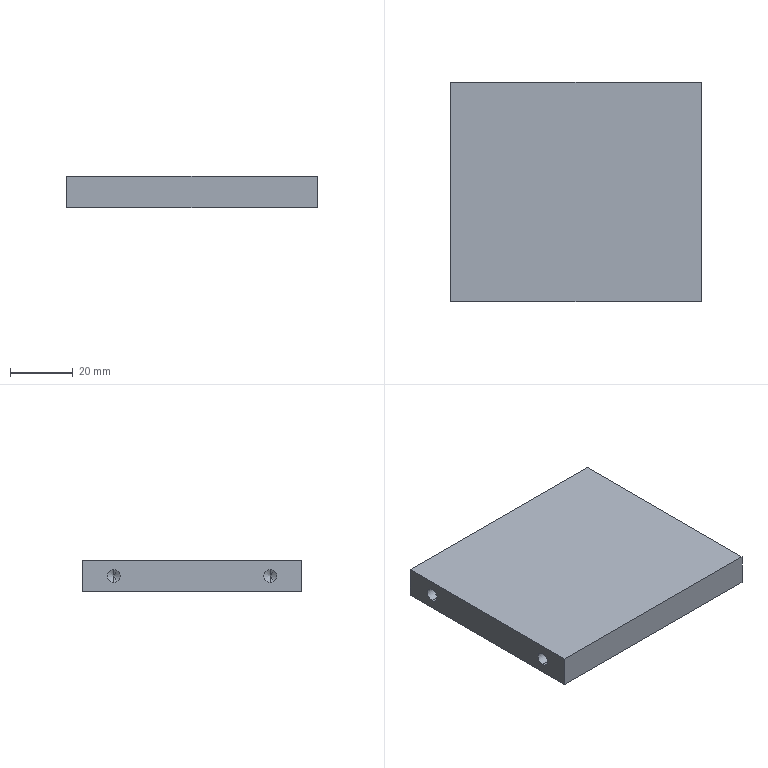Part | SolidWorks | features HoleWzd 2, Extrusion 1 | 1 solid | 22 faces | box 80 x 70 x 10 mm | volume 55201 mm3 | cylinder 8 | cone 8 | plane 6 | commonest cylinder face diameters 4.2 x8
STEP:
#1=CARTESIAN_POINT('',(-26.,25.,2.9));
#2=VERTEX_POINT('',#1);
#3=CARTESIAN_POINT('',(-26.,25.,7.1));
#4=VERTEX_POINT('',#3);
#5=CARTESIAN_POINT('',(-26.,25.,5.));
#6=DIRECTION('',(-1.,0.,0.));
#7=DIRECTION('',(0.,0.,1.));
#8=AXIS2_PLACEMENT_3D('',#5,#6,#7);
#9=CIRCLE('',#8,2.1);
#10=EDGE_CURVE('',#2,#4,#9,.T.);
#11=ORIENTED_EDGE('',*,*,#10,.F.);
#12=CARTESIAN_POINT('',(-40.,25.,2.9));
#13=VERTEX_POINT('',#12);
#14=CARTESIAN_POINT('',(-40.,25.,2.9));
#15=DIRECTION('',(-1.,0.,0.));
#16=VECTOR('',#15,1000.);
#17=LINE('',#14,#16);
#18=EDGE_CURVE('',#2,#13,#17,.T.);
#19=ORIENTED_EDGE('',*,*,#18,.T.);
#20=CARTESIAN_POINT('',(-40.,25.,7.1));
#21=VERTEX_POINT('',#20);
#22=CARTESIAN_POINT('',(-40.,25.,5.));
#23=DIRECTION('',(-1.,0.,0.));
#24=DIRECTION('',(0.,0.,1.));
#25=AXIS2_PLACEMENT_3D('',#22,#23,#24);
#26=CIRCLE('',#25,2.1);
#27=EDGE_CURVE('',#13,#21,#26,.T.);
#28=ORIENTED_EDGE('',*,*,#27,.T.);
#29=CARTESIAN_POINT('',(-40.,25.,7.1));
#30=DIRECTION('',(-1.,0.,0.));
#31=VECTOR('',#30,1000.);
#32=LINE('',#29,#31);
#33=EDGE_CURVE('',#4,#21,#32,.T.);
#34=ORIENTED_EDGE('',*,*,#33,.F.);
#35=EDGE_LOOP('',(#11,#19,#28,#34));
#36=FACE_OUTER_BOUND('',#35,.T.);
#37=CARTESIAN_POINT('',(-40.,25.,5.));
#38=DIRECTION('',(-1.,0.,0.));
#39=DIRECTION('',(0.,0.,1.));
#40=AXIS2_PLACEMENT_3D('',#37,#38,#39);
#41=CYLINDRICAL_SURFACE('',#40,2.1);
#42=ADVANCED_FACE('',(#36),#41,.F.);
#43=CARTESIAN_POINT('',(-24.738,25.,5.));
#44=VERTEX_POINT('',#43);
#45=CARTESIAN_POINT('',(-26.,25.,7.1));
#46=DIRECTION('',(-0.515,0.,0.8572));
#47=VECTOR('',#46,1000.);
#48=LINE('',#45,#47);
#49=EDGE_CURVE('',#44,#4,#48,.T.);
#50=ORIENTED_EDGE('',*,*,#49,.F.);
#51=CARTESIAN_POINT('',(-26.,25.,2.9));
#52=DIRECTION('',(-0.515,0.,-0.8572));
#53=VECTOR('',#52,1000.);
#54=LINE('',#51,#53);
#55=EDGE_CURVE('',#44,#2,#54,.T.);
#56=ORIENTED_EDGE('',*,*,#55,.T.);
#57=ORIENTED_EDGE('',*,*,#10,.T.);
#58=EDGE_LOOP('',(#50,#56,#57));
#59=FACE_OUTER_BOUND('',#58,.T.);
#60=CARTESIAN_POINT('',(-26.,25.,5.));
#61=DIRECTION('',(-1.,0.,0.));
#62=DIRECTION('',(0.,0.,1.));
#63=AXIS2_PLACEMENT_3D('',#60,#61,#62);
#64=CONICAL_SURFACE('',#63,2.1,1.03);
#65=ADVANCED_FACE('',(#59),#64,.F.);
#66=CARTESIAN_POINT('',(-26.,-25.,2.9));
#67=VERTEX_POINT('',#66);
#68=CARTESIAN_POINT('',(-26.,-25.,7.1));
#69=VERTEX_POINT('',#68);
#70=CARTESIAN_POINT('',(-26.,-25.,5.));
#71=DIRECTION('',(-1.,0.,0.));
#72=DIRECTION('',(0.,0.,1.));
#73=AXIS2_PLACEMENT_3D('',#70,#71,#72);
#74=CIRCLE('',#73,2.1);
#75=EDGE_CURVE('',#67,#69,#74,.T.);
#76=ORIENTED_EDGE('',*,*,#75,.F.);
#77=CARTESIAN_POINT('',(-40.,-25.,2.9));
#78=VERTEX_POINT('',#77);
#79=CARTESIAN_POINT('',(-40.,-25.,2.9));
#80=DIRECTION('',(-1.,0.,0.));
#81=VECTOR('',#80,1000.);
#82=LINE('',#79,#81);
#83=EDGE_CURVE('',#67,#78,#82,.T.);
#84=ORIENTED_EDGE('',*,*,#83,.T.);
#85=CARTESIAN_POINT('',(-40.,-25.,7.1));
#86=VERTEX_POINT('',#85);
#87=CARTESIAN_POINT('',(-40.,-25.,5.));
#88=DIRECTION('',(-1.,0.,0.));
#89=DIRECTION('',(0.,0.,1.));
#90=AXIS2_PLACEMENT_3D('',#87,#88,#89);
#91=CIRCLE('',#90,2.1);
#92=EDGE_CURVE('',#78,#86,#91,.T.);
#93=ORIENTED_EDGE('',*,*,#92,.T.);
#94=CARTESIAN_POINT('',(-40.,-25.,7.1));
#95=DIRECTION('',(-1.,0.,0.));
#96=VECTOR('',#95,1000.);
#97=LINE('',#94,#96);
#98=EDGE_CURVE('',#69,#86,#97,.T.);
#99=ORIENTED_EDGE('',*,*,#98,.F.);
#100=EDGE_LOOP('',(#76,#84,#93,#99));
#101=FACE_OUTER_BOUND('',#100,.T.);
#102=CARTESIAN_POINT('',(-40.,-25.,5.));
#103=DIRECTION('',(-1.,0.,0.));
#104=DIRECTION('',(0.,0.,1.));
#105=AXIS2_PLACEMENT_3D('',#102,#103,#104);
#106=CYLINDRICAL_SURFACE('',#105,2.1);
#107=ADVANCED_FACE('',(#101),#106,.F.);
#108=CARTESIAN_POINT('',(-24.738,-25.,5.));
#109=VERTEX_POINT('',#108);
#110=CARTESIAN_POINT('',(-26.,-25.,7.1));
#111=DIRECTION('',(-0.515,0.,0.8572));
#112=VECTOR('',#111,1000.);
#113=LINE('',#110,#112);
#114=EDGE_CURVE('',#109,#69,#113,.T.);
#115=ORIENTED_EDGE('',*,*,#114,.F.);
#116=CARTESIAN_POINT('',(-26.,-25.,2.9));
#117=DIRECTION('',(-0.515,0.,-0.8572));
#118=VECTOR('',#117,1000.);
#119=LINE('',#116,#118);
#120=EDGE_CURVE('',#109,#67,#119,.T.);
#121=ORIENTED_EDGE('',*,*,#120,.T.);
#122=ORIENTED_EDGE('',*,*,#75,.T.);
#123=EDGE_LOOP('',(#115,#121,#122));
#124=FACE_OUTER_BOUND('',#123,.T.);
#125=CARTESIAN_POINT('',(-26.,-25.,5.));
#126=DIRECTION('',(-1.,0.,0.));
#127=DIRECTION('',(0.,0.,1.));
#128=AXIS2_PLACEMENT_3D('',#125,#126,#127);
#129=CONICAL_SURFACE('',#128,2.1,1.03);
#130=ADVANCED_FACE('',(#124),#129,.F.);
#131=CARTESIAN_POINT('',(26.,-25.,7.1));
#132=VERTEX_POINT('',#131);
#133=CARTESIAN_POINT('',(26.,-25.,2.9));
#134=VERTEX_POINT('',#133);
#135=CARTESIAN_POINT('',(26.,-25.,5.));
#136=DIRECTION('',(1.,0.,0.));
#137=DIRECTION('',(0.,0.,-1.));
#138=AXIS2_PLACEMENT_3D('',#135,#136,#137);
#139=CIRCLE('',#138,2.1);
#140=EDGE_CURVE('',#132,#134,#139,.T.);
#141=ORIENTED_EDGE('',*,*,#140,.F.);
#142=CARTESIAN_POINT('',(40.,-25.,7.1));
#143=VERTEX_POINT('',#142);
#144=CARTESIAN_POINT('',(40.,-25.,7.1));
#145=DIRECTION('',(1.,0.,0.));
#146=VECTOR('',#145,1000.);
#147=LINE('',#144,#146);
#148=EDGE_CURVE('',#132,#143,#147,.T.);
#149=ORIENTED_EDGE('',*,*,#148,.T.);
#150=CARTESIAN_POINT('',(40.,-25.,2.9));
#151=VERTEX_POINT('',#150);
#152=CARTESIAN_POINT('',(40.,-25.,5.));
#153=DIRECTION('',(1.,0.,0.));
#154=DIRECTION('',(0.,0.,-1.));
#155=AXIS2_PLACEMENT_3D('',#152,#153,#154);
#156=CIRCLE('',#155,2.1);
#157=EDGE_CURVE('',#143,#151,#156,.T.);
#158=ORIENTED_EDGE('',*,*,#157,.T.);
#159=CARTESIAN_POINT('',(40.,-25.,2.9));
#160=DIRECTION('',(1.,0.,0.));
#161=VECTOR('',#160,1000.);
#162=LINE('',#159,#161);
#163=EDGE_CURVE('',#134,#151,#162,.T.);
#164=ORIENTED_EDGE('',*,*,#163,.F.);
#165=EDGE_LOOP('',(#141,#149,#158,#164));
#166=FACE_OUTER_BOUND('',#165,.T.);
#167=CARTESIAN_POINT('',(40.,-25.,5.));
#168=DIRECTION('',(1.,0.,0.));
#169=DIRECTION('',(0.,0.,-1.));
#170=AXIS2_PLACEMENT_3D('',#167,#168,#169);
#171=CYLINDRICAL_SURFACE('',#170,2.1);
#172=ADVANCED_FACE('',(#166),#171,.F.);
#173=CARTESIAN_POINT('',(24.738,-25.,5.));
#174=VERTEX_POINT('',#173);
#175=CARTESIAN_POINT('',(26.,-25.,2.9));
#176=DIRECTION('',(0.515,0.,-0.8572));
#177=VECTOR('',#176,1000.);
#178=LINE('',#175,#177);
#179=EDGE_CURVE('',#174,#134,#178,.T.);
#180=ORIENTED_EDGE('',*,*,#179,.F.);
#181=CARTESIAN_POINT('',(26.,-25.,7.1));
#182=DIRECTION('',(0.515,0.,0.8572));
#183=VECTOR('',#182,1000.);
#184=LINE('',#181,#183);
#185=EDGE_CURVE('',#174,#132,#184,.T.);
#186=ORIENTED_EDGE('',*,*,#185,.T.);
#187=ORIENTED_EDGE('',*,*,#140,.T.);
#188=EDGE_LOOP('',(#180,#186,#187));
#189=FACE_OUTER_BOUND('',#188,.T.);
#190=CARTESIAN_POINT('',(26.,-25.,5.));
#191=DIRECTION('',(1.,0.,0.));
#192=DIRECTION('',(0.,0.,-1.));
#193=AXIS2_PLACEMENT_3D('',#190,#191,#192);
#194=CONICAL_SURFACE('',#193,2.1,1.03);
#195=ADVANCED_FACE('',(#189),#194,.F.);
#196=CARTESIAN_POINT('',(26.,25.,7.1));
#197=VERTEX_POINT('',#196);
#198=CARTESIAN_POINT('',(26.,25.,2.9));
#199=VERTEX_POINT('',#198);
#200=CARTESIAN_POINT('',(26.,25.,5.));
#201=DIRECTION('',(1.,0.,0.));
#202=DIRECTION('',(0.,0.,-1.));
#203=AXIS2_PLACEMENT_3D('',#200,#201,#202);
#204=CIRCLE('',#203,2.1);
#205=EDGE_CURVE('',#197,#199,#204,.T.);
#206=ORIENTED_EDGE('',*,*,#205,.F.);
#207=CARTESIAN_POINT('',(40.,25.,7.1));
#208=VERTEX_POINT('',#207);
#209=CARTESIAN_POINT('',(40.,25.,7.1));
#210=DIRECTION('',(1.,0.,0.));
#211=VECTOR('',#210,1000.);
#212=LINE('',#209,#211);
#213=EDGE_CURVE('',#197,#208,#212,.T.);
#214=ORIENTED_EDGE('',*,*,#213,.T.);
#215=CARTESIAN_POINT('',(40.,25.,2.9));
#216=VERTEX_POINT('',#215);
#217=CARTESIAN_POINT('',(40.,25.,5.));
#218=DIRECTION('',(1.,0.,0.));
#219=DIRECTION('',(0.,0.,-1.));
#220=AXIS2_PLACEMENT_3D('',#217,#218,#219);
#221=CIRCLE('',#220,2.1);
#222=EDGE_CURVE('',#208,#216,#221,.T.);
#223=ORIENTED_EDGE('',*,*,#222,.T.);
#224=CARTESIAN_POINT('',(40.,25.,2.9));
#225=DIRECTION('',(1.,0.,0.));
#226=VECTOR('',#225,1000.);
#227=LINE('',#224,#226);
#228=EDGE_CURVE('',#199,#216,#227,.T.);
#229=ORIENTED_EDGE('',*,*,#228,.F.);
#230=EDGE_LOOP('',(#206,#214,#223,#229));
#231=FACE_OUTER_BOUND('',#230,.T.);
#232=CARTESIAN_POINT('',(40.,25.,5.));
#233=DIRECTION('',(1.,0.,0.));
#234=DIRECTION('',(0.,0.,-1.));
#235=AXIS2_PLACEMENT_3D('',#232,#233,#234);
#236=CYLINDRICAL_SURFACE('',#235,2.1);
#237=ADVANCED_FACE('',(#231),#236,.F.);
#238=CARTESIAN_POINT('',(24.738,25.,5.));
#239=VERTEX_POINT('',#238);
#240=CARTESIAN_POINT('',(26.,25.,2.9));
#241=DIRECTION('',(0.515,0.,-0.8572));
#242=VECTOR('',#241,1000.);
#243=LINE('',#240,#242);
#244=EDGE_CURVE('',#239,#199,#243,.T.);
#245=ORIENTED_EDGE('',*,*,#244,.F.);
#246=CARTESIAN_POINT('',(26.,25.,7.1));
#247=DIRECTION('',(0.515,0.,0.8572));
#248=VECTOR('',#247,1000.);
#249=LINE('',#246,#248);
#250=EDGE_CURVE('',#239,#197,#249,.T.);
#251=ORIENTED_EDGE('',*,*,#250,.T.);
#252=ORIENTED_EDGE('',*,*,#205,.T.);
#253=EDGE_LOOP('',(#245,#251,#252));
#254=FACE_OUTER_BOUND('',#253,.T.);
#255=CARTESIAN_POINT('',(26.,25.,5.));
#256=DIRECTION('',(1.,0.,0.));
#257=DIRECTION('',(0.,0.,-1.));
#258=AXIS2_PLACEMENT_3D('',#255,#256,#257);
#259=CONICAL_SURFACE('',#258,2.1,1.03);
#260=ADVANCED_FACE('',(#254),#259,.F.);
#261=CARTESIAN_POINT('',(40.,-25.,5.));
#262=DIRECTION('',(1.,0.,0.));
#263=DIRECTION('',(0.,0.,-1.));
#264=AXIS2_PLACEMENT_3D('',#261,#262,#263);
#265=CIRCLE('',#264,2.1);
#266=EDGE_CURVE('',#151,#143,#265,.T.);
#267=ORIENTED_EDGE('',*,*,#266,.F.);
#268=ORIENTED_EDGE('',*,*,#157,.F.);
#269=EDGE_LOOP('',(#267,#268));
#270=FACE_BOUND('',#269,.T.);
#271=CARTESIAN_POINT('',(40.,25.,5.));
#272=DIRECTION('',(1.,0.,0.));
#273=DIRECTION('',(0.,0.,-1.));
#274=AXIS2_PLACEMENT_3D('',#271,#272,#273);
#275=CIRCLE('',#274,2.1);
#276=EDGE_CURVE('',#216,#208,#275,.T.);
#277=ORIENTED_EDGE('',*,*,#276,.F.);
#278=ORIENTED_EDGE('',*,*,#222,.F.);
#279=EDGE_LOOP('',(#277,#278));
#280=FACE_BOUND('',#279,.T.);
#281=CARTESIAN_POINT('',(40.,-35.,0.));
#282=VERTEX_POINT('',#281);
#283=CARTESIAN_POINT('',(40.,35.,0.));
#284=VERTEX_POINT('',#283);
#285=CARTESIAN_POINT('',(40.,35.,0.));
#286=DIRECTION('',(0.,1.,0.));
#287=VECTOR('',#286,1000.);
#288=LINE('',#285,#287);
#289=EDGE_CURVE('',#282,#284,#288,.T.);
#290=ORIENTED_EDGE('',*,*,#289,.T.);
#291=CARTESIAN_POINT('',(40.,35.,10.));
#292=VERTEX_POINT('',#291);
#293=CARTESIAN_POINT('',(40.,35.,10.));
#294=DIRECTION('',(0.,0.,-1.));
#295=VECTOR('',#294,1000.);
#296=LINE('',#293,#295);
#297=EDGE_CURVE('',#292,#284,#296,.T.);
#298=ORIENTED_EDGE('',*,*,#297,.F.);
#299=CARTESIAN_POINT('',(40.,-35.,10.));
#300=VERTEX_POINT('',#299);
#301=CARTESIAN_POINT('',(40.,35.,10.));
#302=DIRECTION('',(0.,1.,0.));
#303=VECTOR('',#302,1000.);
#304=LINE('',#301,#303);
#305=EDGE_CURVE('',#300,#292,#304,.T.);
#306=ORIENTED_EDGE('',*,*,#305,.F.);
#307=CARTESIAN_POINT('',(40.,-35.,10.));
#308=DIRECTION('',(0.,0.,-1.));
#309=VECTOR('',#308,1000.);
#310=LINE('',#307,#309);
#311=EDGE_CURVE('',#300,#282,#310,.T.);
#312=ORIENTED_EDGE('',*,*,#311,.T.);
#313=EDGE_LOOP('',(#290,#298,#306,#312));
#314=FACE_OUTER_BOUND('',#313,.T.);
#315=CARTESIAN_POINT('',(40.,35.,10.));
#316=DIRECTION('',(-1.,0.,0.));
#317=DIRECTION('',(0.,-1.,0.));
#318=AXIS2_PLACEMENT_3D('',#315,#316,#317);
#319=PLANE('',#318);
#320=ADVANCED_FACE('',(#270,#280,#314),#319,.F.);
#321=CARTESIAN_POINT('',(-40.,35.,0.));
#322=VERTEX_POINT('',#321);
#323=CARTESIAN_POINT('',(-40.,35.,0.));
#324=DIRECTION('',(-1.,0.,0.));
#325=VECTOR('',#324,1000.);
#326=LINE('',#323,#325);
#327=EDGE_CURVE('',#284,#322,#326,.T.);
#328=ORIENTED_EDGE('',*,*,#327,.T.);
#329=CARTESIAN_POINT('',(-40.,35.,10.));
#330=VERTEX_POINT('',#329);
#331=CARTESIAN_POINT('',(-40.,35.,10.));
#332=DIRECTION('',(0.,0.,-1.));
#333=VECTOR('',#332,1000.);
#334=LINE('',#331,#333);
#335=EDGE_CURVE('',#330,#322,#334,.T.);
#336=ORIENTED_EDGE('',*,*,#335,.F.);
#337=CARTESIAN_POINT('',(-40.,35.,10.));
#338=DIRECTION('',(-1.,0.,0.));
#339=VECTOR('',#338,1000.);
#340=LINE('',#337,#339);
#341=EDGE_CURVE('',#292,#330,#340,.T.);
#342=ORIENTED_EDGE('',*,*,#341,.F.);
#343=ORIENTED_EDGE('',*,*,#297,.T.);
#344=EDGE_LOOP('',(#328,#336,#342,#343));
#345=FACE_OUTER_BOUND('',#344,.T.);
#346=CARTESIAN_POINT('',(-40.,35.,10.));
#347=DIRECTION('',(0.,-1.,0.));
#348=DIRECTION('',(0.,0.,-1.));
#349=AXIS2_PLACEMENT_3D('',#346,#347,#348);
#350=PLANE('',#349);
#351=ADVANCED_FACE('',(#345),#350,.F.);
#352=CARTESIAN_POINT('',(-40.,25.,5.));
#353=DIRECTION('',(-1.,0.,0.));
#354=DIRECTION('',(0.,0.,1.));
#355=AXIS2_PLACEMENT_3D('',#352,#353,#354);
#356=CIRCLE('',#355,2.1);
#357=EDGE_CURVE('',#21,#13,#356,.T.);
#358=ORIENTED_EDGE('',*,*,#357,.F.);
#359=ORIENTED_EDGE('',*,*,#27,.F.);
#360=EDGE_LOOP('',(#358,#359));
#361=FACE_BOUND('',#360,.T.);
#362=CARTESIAN_POINT('',(-40.,-25.,5.));
#363=DIRECTION('',(-1.,0.,0.));
#364=DIRECTION('',(0.,0.,1.));
#365=AXIS2_PLACEMENT_3D('',#362,#363,#364);
#366=CIRCLE('',#365,2.1);
#367=EDGE_CURVE('',#86,#78,#366,.T.);
#368=ORIENTED_EDGE('',*,*,#367,.F.);
#369=ORIENTED_EDGE('',*,*,#92,.F.);
#370=EDGE_LOOP('',(#368,#369));
#371=FACE_BOUND('',#370,.T.);
#372=CARTESIAN_POINT('',(-40.,-35.,0.));
#373=VERTEX_POINT('',#372);
#374=CARTESIAN_POINT('',(-40.,35.,0.));
#375=DIRECTION('',(0.,-1.,0.));
#376=VECTOR('',#375,1000.);
#377=LINE('',#374,#376);
#378=EDGE_CURVE('',#322,#373,#377,.T.);
#379=ORIENTED_EDGE('',*,*,#378,.T.);
#380=CARTESIAN_POINT('',(-40.,-35.,10.));
#381=VERTEX_POINT('',#380);
#382=CARTESIAN_POINT('',(-40.,-35.,10.));
#383=DIRECTION('',(0.,0.,-1.));
#384=VECTOR('',#383,1000.);
#385=LINE('',#382,#384);
#386=EDGE_CURVE('',#381,#373,#385,.T.);
#387=ORIENTED_EDGE('',*,*,#386,.F.);
#388=CARTESIAN_POINT('',(-40.,35.,10.));
#389=DIRECTION('',(0.,-1.,0.));
#390=VECTOR('',#389,1000.);
#391=LINE('',#388,#390);
#392=EDGE_CURVE('',#330,#381,#391,.T.);
#393=ORIENTED_EDGE('',*,*,#392,.F.);
#394=ORIENTED_EDGE('',*,*,#335,.T.);
#395=EDGE_LOOP('',(#379,#387,#393,#394));
#396=FACE_OUTER_BOUND('',#395,.T.);
#397=CARTESIAN_POINT('',(-40.,35.,10.));
#398=DIRECTION('',(1.,0.,0.));
#399=DIRECTION('',(0.,1.,0.));
#400=AXIS2_PLACEMENT_3D('',#397,#398,#399);
#401=PLANE('',#400);
#402=ADVANCED_FACE('',(#361,#371,#396),#401,.F.);
#403=CARTESIAN_POINT('',(-40.,-35.,0.));
#404=DIRECTION('',(1.,0.,0.));
#405=VECTOR('',#404,1000.);
#406=LINE('',#403,#405);
#407=EDGE_CURVE('',#373,#282,#406,.T.);
#408=ORIENTED_EDGE('',*,*,#407,.T.);
#409=ORIENTED_EDGE('',*,*,#311,.F.);
#410=CARTESIAN_POINT('',(-40.,-35.,10.));
#411=DIRECTION('',(1.,0.,0.));
#412=VECTOR('',#411,1000.);
#413=LINE('',#410,#412);
#414=EDGE_CURVE('',#381,#300,#413,.T.);
#415=ORIENTED_EDGE('',*,*,#414,.F.);
#416=ORIENTED_EDGE('',*,*,#386,.T.);
#417=EDGE_LOOP('',(#408,#409,#415,#416));
#418=FACE_OUTER_BOUND('',#417,.T.);
#419=CARTESIAN_POINT('',(-40.,-35.,10.));
#420=DIRECTION('',(0.,1.,0.));
#421=DIRECTION('',(0.,0.,1.));
#422=AXIS2_PLACEMENT_3D('',#419,#420,#421);
#423=PLANE('',#422);
#424=ADVANCED_FACE('',(#418),#423,.F.);
#425=ORIENTED_EDGE('',*,*,#305,.T.);
#426=ORIENTED_EDGE('',*,*,#341,.T.);
#427=ORIENTED_EDGE('',*,*,#392,.T.);
#428=ORIENTED_EDGE('',*,*,#414,.T.);
#429=EDGE_LOOP('',(#425,#426,#427,#428));
#430=FACE_OUTER_BOUND('',#429,.T.);
#431=CARTESIAN_POINT('',(0.,0.,10.));
#432=DIRECTION('',(0.,0.,1.));
#433=DIRECTION('',(1.,0.,0.));
#434=AXIS2_PLACEMENT_3D('',#431,#432,#433);
#435=PLANE('',#434);
#436=ADVANCED_FACE('',(#430),#435,.T.);
#437=ORIENTED_EDGE('',*,*,#289,.F.);
#438=ORIENTED_EDGE('',*,*,#407,.F.);
#439=ORIENTED_EDGE('',*,*,#378,.F.);
#440=ORIENTED_EDGE('',*,*,#327,.F.);
#441=EDGE_LOOP('',(#437,#438,#439,#440));
#442=FACE_OUTER_BOUND('',#441,.T.);
#443=CARTESIAN_POINT('',(0.,0.,0.));
#444=DIRECTION('',(0.,0.,1.));
#445=DIRECTION('',(1.,0.,0.));
#446=AXIS2_PLACEMENT_3D('',#443,#444,#445);
#447=PLANE('',#446);
#448=ADVANCED_FACE('',(#442),#447,.F.);
#449=ORIENTED_EDGE('',*,*,#250,.F.);
#450=ORIENTED_EDGE('',*,*,#244,.T.);
#451=CARTESIAN_POINT('',(26.,25.,5.));
#452=DIRECTION('',(1.,0.,0.));
#453=DIRECTION('',(0.,0.,-1.));
#454=AXIS2_PLACEMENT_3D('',#451,#452,#453);
#455=CIRCLE('',#454,2.1);
#456=EDGE_CURVE('',#199,#197,#455,.T.);
#457=ORIENTED_EDGE('',*,*,#456,.T.);
#458=EDGE_LOOP('',(#449,#450,#457));
#459=FACE_OUTER_BOUND('',#458,.T.);
#460=CARTESIAN_POINT('',(26.,25.,5.));
#461=DIRECTION('',(1.,0.,0.));
#462=DIRECTION('',(0.,0.,-1.));
#463=AXIS2_PLACEMENT_3D('',#460,#461,#462);
#464=CONICAL_SURFACE('',#463,2.1,1.03);
#465=ADVANCED_FACE('',(#459),#464,.F.);
#466=ORIENTED_EDGE('',*,*,#213,.F.);
#467=ORIENTED_EDGE('',*,*,#456,.F.);
#468=ORIENTED_EDGE('',*,*,#228,.T.);
#469=ORIENTED_EDGE('',*,*,#276,.T.);
#470=EDGE_LOOP('',(#466,#467,#468,#469));
#471=FACE_OUTER_BOUND('',#470,.T.);
#472=CARTESIAN_POINT('',(40.,25.,5.));
#473=DIRECTION('',(1.,0.,0.));
#474=DIRECTION('',(0.,0.,-1.));
#475=AXIS2_PLACEMENT_3D('',#472,#473,#474);
#476=CYLINDRICAL_SURFACE('',#475,2.1);
#477=ADVANCED_FACE('',(#471),#476,.F.);
#478=ORIENTED_EDGE('',*,*,#185,.F.);
#479=ORIENTED_EDGE('',*,*,#179,.T.);
#480=CARTESIAN_POINT('',(26.,-25.,5.));
#481=DIRECTION('',(1.,0.,0.));
#482=DIRECTION('',(0.,0.,-1.));
#483=AXIS2_PLACEMENT_3D('',#480,#481,#482);
#484=CIRCLE('',#483,2.1);
#485=EDGE_CURVE('',#134,#132,#484,.T.);
#486=ORIENTED_EDGE('',*,*,#485,.T.);
#487=EDGE_LOOP('',(#478,#479,#486));
#488=FACE_OUTER_BOUND('',#487,.T.);
#489=CARTESIAN_POINT('',(26.,-25.,5.));
#490=DIRECTION('',(1.,0.,0.));
#491=DIRECTION('',(0.,0.,-1.));
#492=AXIS2_PLACEMENT_3D('',#489,#490,#491);
#493=CONICAL_SURFACE('',#492,2.1,1.03);
#494=ADVANCED_FACE('',(#488),#493,.F.);
#495=ORIENTED_EDGE('',*,*,#148,.F.);
#496=ORIENTED_EDGE('',*,*,#485,.F.);
#497=ORIENTED_EDGE('',*,*,#163,.T.);
#498=ORIENTED_EDGE('',*,*,#266,.T.);
#499=EDGE_LOOP('',(#495,#496,#497,#498));
#500=FACE_OUTER_BOUND('',#499,.T.);
#501=CARTESIAN_POINT('',(40.,-25.,5.));
#502=DIRECTION('',(1.,0.,0.));
#503=DIRECTION('',(0.,0.,-1.));
#504=AXIS2_PLACEMENT_3D('',#501,#502,#503);
#505=CYLINDRICAL_SURFACE('',#504,2.1);
#506=ADVANCED_FACE('',(#500),#505,.F.);
#507=ORIENTED_EDGE('',*,*,#120,.F.);
#508=ORIENTED_EDGE('',*,*,#114,.T.);
#509=CARTESIAN_POINT('',(-26.,-25.,5.));
#510=DIRECTION('',(-1.,0.,0.));
#511=DIRECTION('',(0.,0.,1.));
#512=AXIS2_PLACEMENT_3D('',#509,#510,#511);
#513=CIRCLE('',#512,2.1);
#514=EDGE_CURVE('',#69,#67,#513,.T.);
#515=ORIENTED_EDGE('',*,*,#514,.T.);
#516=EDGE_LOOP('',(#507,#508,#515));
#517=FACE_OUTER_BOUND('',#516,.T.);
#518=CARTESIAN_POINT('',(-26.,-25.,5.));
#519=DIRECTION('',(-1.,0.,0.));
#520=DIRECTION('',(0.,0.,1.));
#521=AXIS2_PLACEMENT_3D('',#518,#519,#520);
#522=CONICAL_SURFACE('',#521,2.1,1.03);
#523=ADVANCED_FACE('',(#517),#522,.F.);
#524=ORIENTED_EDGE('',*,*,#83,.F.);
#525=ORIENTED_EDGE('',*,*,#514,.F.);
#526=ORIENTED_EDGE('',*,*,#98,.T.);
#527=ORIENTED_EDGE('',*,*,#367,.T.);
#528=EDGE_LOOP('',(#524,#525,#526,#527));
#529=FACE_OUTER_BOUND('',#528,.T.);
#530=CARTESIAN_POINT('',(-40.,-25.,5.));
#531=DIRECTION('',(-1.,0.,0.));
#532=DIRECTION('',(0.,0.,1.));
#533=AXIS2_PLACEMENT_3D('',#530,#531,#532);
#534=CYLINDRICAL_SURFACE('',#533,2.1);
#535=ADVANCED_FACE('',(#529),#534,.F.);
#536=ORIENTED_EDGE('',*,*,#55,.F.);
#537=ORIENTED_EDGE('',*,*,#49,.T.);
#538=CARTESIAN_POINT('',(-26.,25.,5.));
#539=DIRECTION('',(-1.,0.,0.));
#540=DIRECTION('',(0.,0.,1.));
#541=AXIS2_PLACEMENT_3D('',#538,#539,#540);
#542=CIRCLE('',#541,2.1);
#543=EDGE_CURVE('',#4,#2,#542,.T.);
#544=ORIENTED_EDGE('',*,*,#543,.T.);
#545=EDGE_LOOP('',(#536,#537,#544));
#546=FACE_OUTER_BOUND('',#545,.T.);
#547=CARTESIAN_POINT('',(-26.,25.,5.));
#548=DIRECTION('',(-1.,0.,0.));
#549=DIRECTION('',(0.,0.,1.));
#550=AXIS2_PLACEMENT_3D('',#547,#548,#549);
#551=CONICAL_SURFACE('',#550,2.1,1.03);
#552=ADVANCED_FACE('',(#546),#551,.F.);
#553=ORIENTED_EDGE('',*,*,#18,.F.);
#554=ORIENTED_EDGE('',*,*,#543,.F.);
#555=ORIENTED_EDGE('',*,*,#33,.T.);
#556=ORIENTED_EDGE('',*,*,#357,.T.);
#557=EDGE_LOOP('',(#553,#554,#555,#556));
#558=FACE_OUTER_BOUND('',#557,.T.);
#559=CARTESIAN_POINT('',(-40.,25.,5.));
#560=DIRECTION('',(-1.,0.,0.));
#561=DIRECTION('',(0.,0.,1.));
#562=AXIS2_PLACEMENT_3D('',#559,#560,#561);
#563=CYLINDRICAL_SURFACE('',#562,2.1);
#564=ADVANCED_FACE('',(#558),#563,.F.);
#565=CLOSED_SHELL('',(#42,#65,#107,#130,#172,#195,#237,#260,#320,#351,#402,#424,#436,#448,#465,#477,#494,#506,#523,#535,#552,#564));
#566=MANIFOLD_SOLID_BREP('',#565);
#567=CARTESIAN_POINT('',(0.,0.,0.));
#568=DIRECTION('',(0.,0.,1.));
#569=DIRECTION('',(1.,0.,0.));
#570=AXIS2_PLACEMENT_3D('',#567,#568,#569);
#571=(LENGTH_UNIT()NAMED_UNIT(*)SI_UNIT(.MILLI.,.METRE.));
#572=UNCERTAINTY_MEASURE_WITH_UNIT(LENGTH_MEASURE(0.00001),#571,'','');
#573=(NAMED_UNIT(*)PLANE_ANGLE_UNIT()SI_UNIT($,.RADIAN.));
#574=(NAMED_UNIT(*)SI_UNIT($,.STERADIAN.)SOLID_ANGLE_UNIT());
#575=(GEOMETRIC_REPRESENTATION_CONTEXT(3)GLOBAL_UNCERTAINTY_ASSIGNED_CONTEXT((#572))GLOBAL_UNIT_ASSIGNED_CONTEXT((#571,#573,#574))REPRESENTATION_CONTEXT('',''));
#576=ADVANCED_BREP_SHAPE_REPRESENTATION('',(#566,#570),#575);